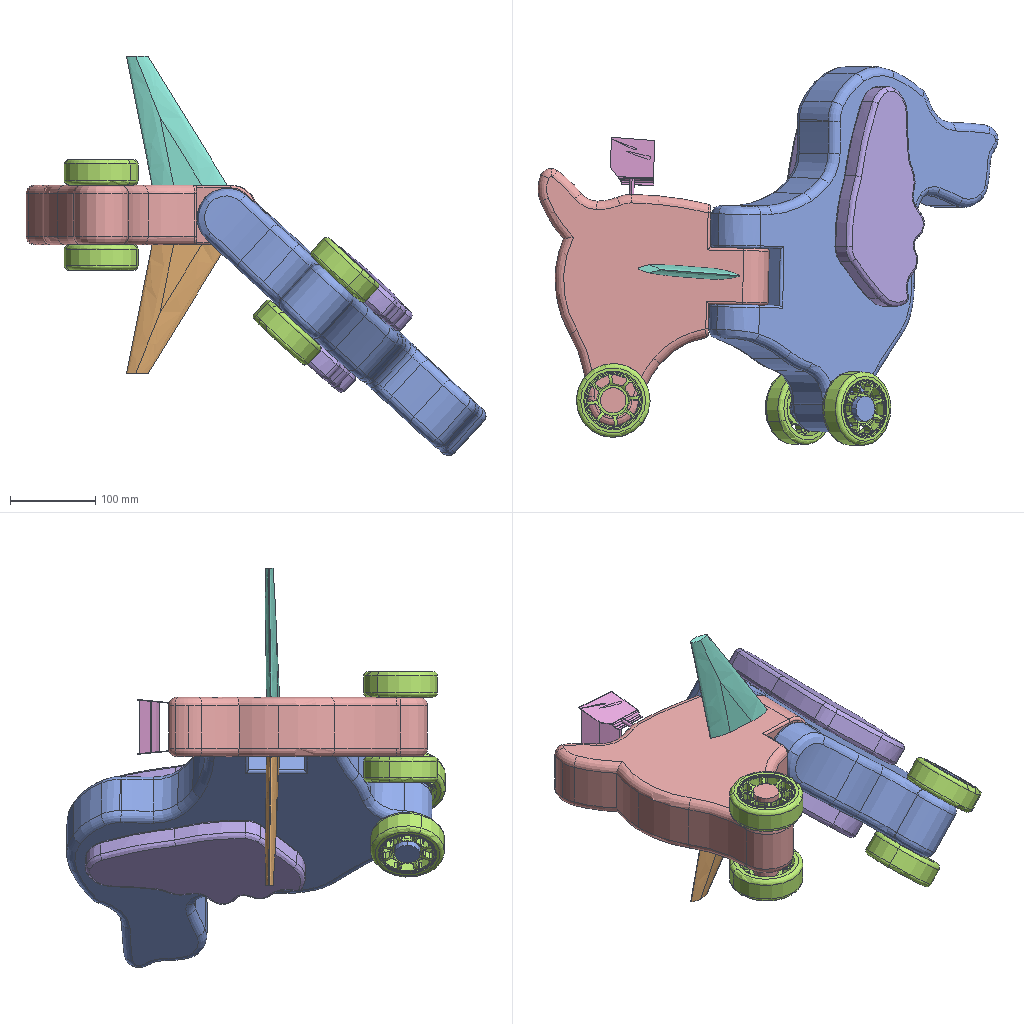Assembly | SolidWorks | 6 different items | 9 placed | box 541 x 446 x 469 mm
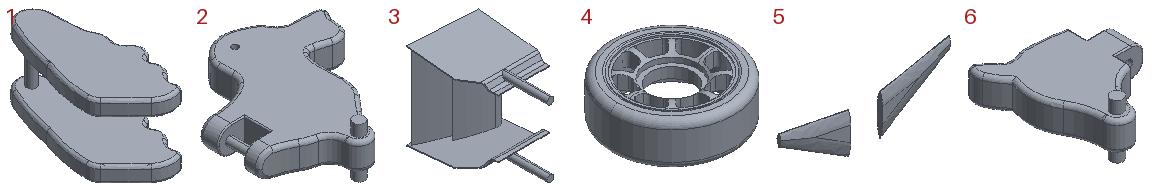Parts list (item | quantity | size | volume | features):
1 | x1 | 124.14 x 258.791 x 126.388 mm | 1203274 mm3 | features Extrusion 1, Fillet 1, ICE 1, MirrorSolid 1
2 | x1 | 416.464 x 430.21 x 130 mm | 5952307 mm3 | features ICE 4, Fillet 3
3 | x1 | 50.8 x 81.634 x 64.383 mm | 11608 mm3 | features ICE 4, Extrusion 1, MirrorSolid 1
4 | x4 | 86.769 x 86.769 x 30 mm | 85929 mm3 | features ICE 3, Fillet 2, Extrusion 1, Revolution 1
5 | x1 | 372.694 x 12.7 x 118.906 mm | 155010 mm3 | features Fillet 4, Extrusion 1, MirrorSolid 1
6 | x1 | 273.069 x 303.303 x 130 mm | 3030227 mm3 | features Fillet 3, ICE 3, Extrusion 1
Mates (type | each side: item.copy, entity, surface, feature):
Concentric | 6.1 face cylinder Boss-Extrude2 | 4.1 face cylinder Revolve2
Coincident | 6.1 face plane Boss-Extrude1 | 4.1 face plane Boss-Extrude1
Coincident | 6.1 face plane Boss-Extrude1 | 2.1 face plane Boss-Extrude2
Concentric | 6.1 face cylinder Cut-Extrude3 | 2.1 face cylinder Boss-Extrude3
Concentric | 6.1 face cylinder Cut-Extrude4 | 3.1 face cylinder Boss-Extrude1
Coincident | 6.1 face plane Cut-Extrude4 | 3.1 face plane Boss-Extrude1
Coincident | 6.1 face plane Boss-Extrude1 | 5.1 face plane Boss-Extrude1
Parallel | 3.1 face plane Cut-Extrude2 | 5.1 face plane Boss-Extrude1
Concentric | 2.1 face cylinder Boss-Extrude4 | 4.2 face cylinder Revolve2
Coincident | 2.1 face plane Boss-Extrude2 | 4.2 face plane Boss-Extrude1
Lock | 6.1 select_type:0 | 5.1 select_type:0
Concentric | 2.1 face cylinder Cut-Extrude1 | 1.1 face cylinder Boss-Extrude2
Coincident | 2.1 face plane Boss-Extrude2 | 1.1 face plane Mirror1
Concentric | 2.1 face cylinder Boss-Extrude4 | 4.3 face cylinder Revolve2
Coincident | 6.1 face plane Boss-Extrude1 | 4.4 face plane Boss-Extrude1
Concentric | 6.1 face cylinder Boss-Extrude2 | 4.4 face cylinder Revolve2
Coincident | 2.1 face plane Boss-Extrude2 | 4.3 face plane Boss-Extrude1